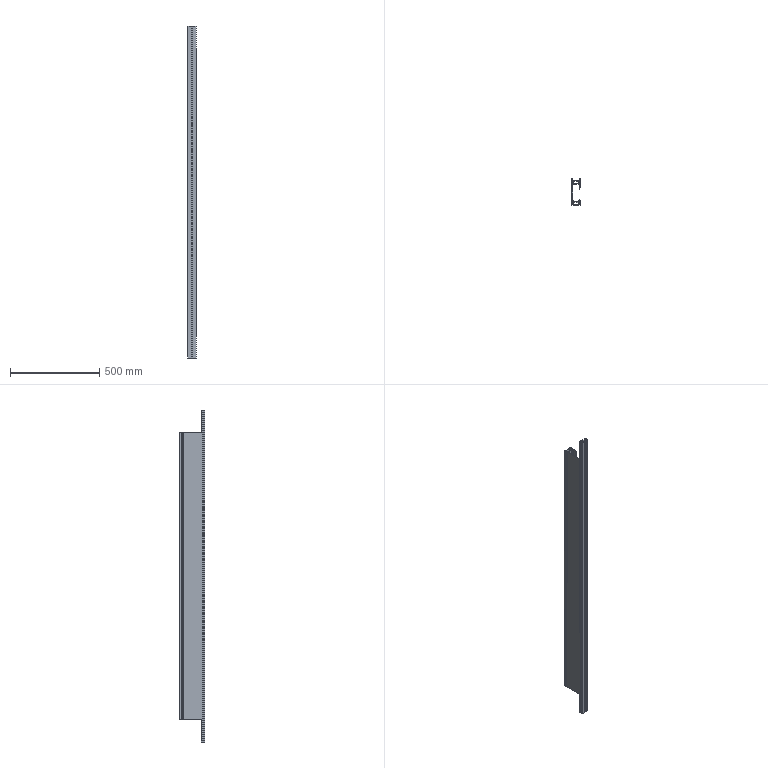Part | SolidWorks | features ICE 10, Fillet 8, MirrorPattern 2, Extrusion 1, LPattern 1 | 1 solid | 118 faces | box 45 x 145 x 1860 mm | volume 2040055 mm3 | plane 111 | cylinder 7 | commonest cylinder face diameters 4 x5 3 x1 20 x1